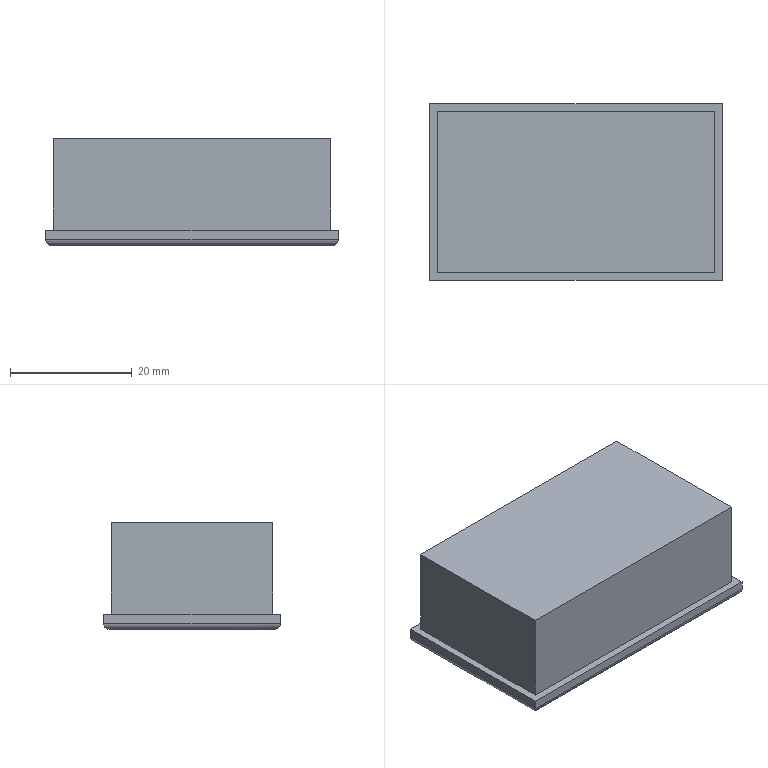Part | SolidWorks | features BaseBody 1 | 1 solid | 27 faces | box 48 x 29 x 17.5 mm | volume 19851 mm3 | plane 23 | cylinder 4 | commonest cylinder face diameters 2 x4
STEP:
#1=CARTESIAN_POINT('',(14.5,-5.,2.));
#2=VERTEX_POINT('',#1);
#3=CARTESIAN_POINT('',(12.5,-5.,2.));
#4=VERTEX_POINT('',#3);
#5=CARTESIAN_POINT('',(0.,-5.,2.));
#6=DIRECTION('',(-1.,0.,0.));
#7=VECTOR('',#6,1000.);
#8=LINE('',#5,#7);
#9=EDGE_CURVE('',#2,#4,#8,.T.);
#10=ORIENTED_EDGE('',*,*,#9,.T.);
#11=CARTESIAN_POINT('',(12.5,5.,2.));
#12=VERTEX_POINT('',#11);
#13=CARTESIAN_POINT('',(12.5,0.,2.));
#14=DIRECTION('',(0.,1.,0.));
#15=VECTOR('',#14,1000.);
#16=LINE('',#13,#15);
#17=EDGE_CURVE('',#4,#12,#16,.T.);
#18=ORIENTED_EDGE('',*,*,#17,.T.);
#19=CARTESIAN_POINT('',(14.5,5.,2.));
#20=VERTEX_POINT('',#19);
#21=CARTESIAN_POINT('',(0.,5.,2.));
#22=DIRECTION('',(1.,0.,0.));
#23=VECTOR('',#22,1000.);
#24=LINE('',#21,#23);
#25=EDGE_CURVE('',#12,#20,#24,.T.);
#26=ORIENTED_EDGE('',*,*,#25,.T.);
#27=CARTESIAN_POINT('',(14.5,0.,2.));
#28=DIRECTION('',(0.,-1.,0.));
#29=VECTOR('',#28,1000.);
#30=LINE('',#27,#29);
#31=EDGE_CURVE('',#20,#2,#30,.T.);
#32=ORIENTED_EDGE('',*,*,#31,.T.);
#33=EDGE_LOOP('',(#10,#18,#26,#32));
#34=FACE_OUTER_BOUND('',#33,.T.);
#35=CARTESIAN_POINT('',(0.,0.,2.));
#36=DIRECTION('',(0.,0.,1.));
#37=DIRECTION('',(1.,0.,0.));
#38=AXIS2_PLACEMENT_3D('',#35,#36,#37);
#39=PLANE('',#38);
#40=ADVANCED_FACE('',(#34),#39,.F.);
#41=CARTESIAN_POINT('',(-21.,11.5,0.));
#42=VERTEX_POINT('',#41);
#43=CARTESIAN_POINT('',(21.,11.5,0.));
#44=VERTEX_POINT('',#43);
#45=CARTESIAN_POINT('',(21.,11.5,0.));
#46=DIRECTION('',(1.,0.,0.));
#47=VECTOR('',#46,1000.);
#48=LINE('',#45,#47);
#49=EDGE_CURVE('',#42,#44,#48,.T.);
#50=ORIENTED_EDGE('',*,*,#49,.T.);
#51=CARTESIAN_POINT('',(19.,9.5,2.));
#52=VERTEX_POINT('',#51);
#53=CARTESIAN_POINT('',(21.,11.5,0.));
#54=DIRECTION('',(0.5774,0.5774,-0.5774));
#55=VECTOR('',#54,1000.);
#56=LINE('',#53,#55);
#57=EDGE_CURVE('',#52,#44,#56,.T.);
#58=ORIENTED_EDGE('',*,*,#57,.F.);
#59=CARTESIAN_POINT('',(-19.,9.5,2.));
#60=VERTEX_POINT('',#59);
#61=CARTESIAN_POINT('',(21.,9.5,2.));
#62=DIRECTION('',(1.,0.,0.));
#63=VECTOR('',#62,1000.);
#64=LINE('',#61,#63);
#65=EDGE_CURVE('',#60,#52,#64,.T.);
#66=ORIENTED_EDGE('',*,*,#65,.F.);
#67=CARTESIAN_POINT('',(-13.333,3.833,7.667));
#68=DIRECTION('',(-0.5774,0.5774,-0.5774));
#69=VECTOR('',#68,1000.);
#70=LINE('',#67,#69);
#71=EDGE_CURVE('',#60,#42,#70,.T.);
#72=ORIENTED_EDGE('',*,*,#71,.T.);
#73=EDGE_LOOP('',(#50,#58,#66,#72));
#74=FACE_OUTER_BOUND('',#73,.T.);
#75=CARTESIAN_POINT('',(21.,11.5,0.));
#76=DIRECTION('',(0.,0.7071,0.7071));
#77=DIRECTION('',(1.,0.,0.));
#78=AXIS2_PLACEMENT_3D('',#75,#76,#77);
#79=PLANE('',#78);
#80=ADVANCED_FACE('',(#74),#79,.F.);
#81=CARTESIAN_POINT('',(21.,-11.5,0.));
#82=VERTEX_POINT('',#81);
#83=CARTESIAN_POINT('',(21.,-11.5,0.));
#84=DIRECTION('',(0.,-1.,0.));
#85=VECTOR('',#84,1000.);
#86=LINE('',#83,#85);
#87=EDGE_CURVE('',#44,#82,#86,.T.);
#88=ORIENTED_EDGE('',*,*,#87,.T.);
#89=CARTESIAN_POINT('',(19.,-9.5,2.));
#90=VERTEX_POINT('',#89);
#91=CARTESIAN_POINT('',(21.,-11.5,0.));
#92=DIRECTION('',(0.5774,-0.5774,-0.5774));
#93=VECTOR('',#92,1000.);
#94=LINE('',#91,#93);
#95=EDGE_CURVE('',#90,#82,#94,.T.);
#96=ORIENTED_EDGE('',*,*,#95,.F.);
#97=CARTESIAN_POINT('',(19.,-11.5,2.));
#98=DIRECTION('',(0.,-1.,0.));
#99=VECTOR('',#98,1000.);
#100=LINE('',#97,#99);
#101=EDGE_CURVE('',#52,#90,#100,.T.);
#102=ORIENTED_EDGE('',*,*,#101,.F.);
#103=ORIENTED_EDGE('',*,*,#57,.T.);
#104=EDGE_LOOP('',(#88,#96,#102,#103));
#105=FACE_OUTER_BOUND('',#104,.T.);
#106=CARTESIAN_POINT('',(21.,-11.5,0.));
#107=DIRECTION('',(0.7071,0.,0.7071));
#108=DIRECTION('',(0.,-1.,0.));
#109=AXIS2_PLACEMENT_3D('',#106,#107,#108);
#110=PLANE('',#109);
#111=ADVANCED_FACE('',(#105),#110,.F.);
#112=CARTESIAN_POINT('',(-21.,-11.5,0.));
#113=VERTEX_POINT('',#112);
#114=CARTESIAN_POINT('',(21.,-11.5,0.));
#115=DIRECTION('',(-1.,0.,0.));
#116=VECTOR('',#115,1000.);
#117=LINE('',#114,#116);
#118=EDGE_CURVE('',#82,#113,#117,.T.);
#119=ORIENTED_EDGE('',*,*,#118,.T.);
#120=CARTESIAN_POINT('',(-19.,-9.5,2.));
#121=VERTEX_POINT('',#120);
#122=CARTESIAN_POINT('',(-7.,2.5,14.));
#123=DIRECTION('',(-0.5774,-0.5774,-0.5774));
#124=VECTOR('',#123,1000.);
#125=LINE('',#122,#124);
#126=EDGE_CURVE('',#121,#113,#125,.T.);
#127=ORIENTED_EDGE('',*,*,#126,.F.);
#128=CARTESIAN_POINT('',(21.,-9.5,2.));
#129=DIRECTION('',(-1.,0.,0.));
#130=VECTOR('',#129,1000.);
#131=LINE('',#128,#130);
#132=EDGE_CURVE('',#90,#121,#131,.T.);
#133=ORIENTED_EDGE('',*,*,#132,.F.);
#134=ORIENTED_EDGE('',*,*,#95,.T.);
#135=EDGE_LOOP('',(#119,#127,#133,#134));
#136=FACE_OUTER_BOUND('',#135,.T.);
#137=CARTESIAN_POINT('',(21.,-11.5,0.));
#138=DIRECTION('',(0.,-0.7071,0.7071));
#139=DIRECTION('',(-1.,0.,0.));
#140=AXIS2_PLACEMENT_3D('',#137,#138,#139);
#141=PLANE('',#140);
#142=ADVANCED_FACE('',(#136),#141,.F.);
#143=CARTESIAN_POINT('',(-21.,-11.5,0.));
#144=DIRECTION('',(0.,1.,0.));
#145=VECTOR('',#144,1000.);
#146=LINE('',#143,#145);
#147=EDGE_CURVE('',#113,#42,#146,.T.);
#148=ORIENTED_EDGE('',*,*,#147,.T.);
#149=ORIENTED_EDGE('',*,*,#71,.F.);
#150=CARTESIAN_POINT('',(-19.,-11.5,2.));
#151=DIRECTION('',(0.,1.,0.));
#152=VECTOR('',#151,1000.);
#153=LINE('',#150,#152);
#154=EDGE_CURVE('',#121,#60,#153,.T.);
#155=ORIENTED_EDGE('',*,*,#154,.F.);
#156=ORIENTED_EDGE('',*,*,#126,.T.);
#157=EDGE_LOOP('',(#148,#149,#155,#156));
#158=FACE_OUTER_BOUND('',#157,.T.);
#159=CARTESIAN_POINT('',(-21.,-11.5,0.));
#160=DIRECTION('',(-0.7071,0.,0.7071));
#161=DIRECTION('',(0.,1.,0.));
#162=AXIS2_PLACEMENT_3D('',#159,#160,#161);
#163=PLANE('',#162);
#164=ADVANCED_FACE('',(#158),#163,.F.);
#165=CARTESIAN_POINT('',(24.,-14.5,1.));
#166=VERTEX_POINT('',#165);
#167=CARTESIAN_POINT('',(23.,-13.5,0.));
#168=VERTEX_POINT('',#167);
#169=CARTESIAN_POINT('',(24.,-14.5,1.));
#170=CARTESIAN_POINT('',(24.,-14.5,0.4142));
#171=CARTESIAN_POINT('',(23.586,-14.086,0.));
#172=CARTESIAN_POINT('',(23.,-13.5,0.));
#173=(BOUNDED_CURVE()B_SPLINE_CURVE(3,(#169,#170,#171,#172),.UNSPECIFIED.,.F.,.T.)B_SPLINE_CURVE_WITH_KNOTS((4,4),(3.142,4.712),.UNSPECIFIED.)CURVE()GEOMETRIC_REPRESENTATION_ITEM()RATIONAL_B_SPLINE_CURVE((1.,0.8047,0.8047,1.))REPRESENTATION_ITEM(''));
#174=EDGE_CURVE('',#166,#168,#173,.T.);
#175=ORIENTED_EDGE('',*,*,#174,.T.);
#176=CARTESIAN_POINT('',(23.,13.5,0.));
#177=VERTEX_POINT('',#176);
#178=CARTESIAN_POINT('',(23.,-14.5,0.));
#179=DIRECTION('',(0.,-1.,0.));
#180=VECTOR('',#179,1000.);
#181=LINE('',#178,#180);
#182=EDGE_CURVE('',#177,#168,#181,.T.);
#183=ORIENTED_EDGE('',*,*,#182,.F.);
#184=CARTESIAN_POINT('',(24.,14.5,1.));
#185=VERTEX_POINT('',#184);
#186=CARTESIAN_POINT('',(23.,13.5,0.));
#187=CARTESIAN_POINT('',(23.586,14.086,0.));
#188=CARTESIAN_POINT('',(24.,14.5,0.4142));
#189=CARTESIAN_POINT('',(24.,14.5,1.));
#190=(BOUNDED_CURVE()B_SPLINE_CURVE(3,(#186,#187,#188,#189),.UNSPECIFIED.,.F.,.F.)B_SPLINE_CURVE_WITH_KNOTS((4,4),(4.712,6.283),.UNSPECIFIED.)CURVE()GEOMETRIC_REPRESENTATION_ITEM()RATIONAL_B_SPLINE_CURVE((1.,0.8047,0.8047,1.))REPRESENTATION_ITEM(''));
#191=EDGE_CURVE('',#177,#185,#190,.T.);
#192=ORIENTED_EDGE('',*,*,#191,.T.);
#193=CARTESIAN_POINT('',(24.,14.5,1.));
#194=DIRECTION('',(0.,1.,0.));
#195=VECTOR('',#194,1000.);
#196=LINE('',#193,#195);
#197=EDGE_CURVE('',#166,#185,#196,.T.);
#198=ORIENTED_EDGE('',*,*,#197,.F.);
#199=EDGE_LOOP('',(#175,#183,#192,#198));
#200=FACE_OUTER_BOUND('',#199,.T.);
#201=CARTESIAN_POINT('',(23.,-14.5,1.));
#202=DIRECTION('',(0.,-1.,0.));
#203=DIRECTION('',(0.,0.,-1.));
#204=AXIS2_PLACEMENT_3D('',#201,#202,#203);
#205=CYLINDRICAL_SURFACE('',#204,1.);
#206=ADVANCED_FACE('',(#200),#205,.T.);
#207=CARTESIAN_POINT('',(-23.,13.5,0.));
#208=VERTEX_POINT('',#207);
#209=CARTESIAN_POINT('',(-24.,14.5,1.));
#210=VERTEX_POINT('',#209);
#211=CARTESIAN_POINT('',(-23.,13.5,0.));
#212=CARTESIAN_POINT('',(-23.586,14.086,0.));
#213=CARTESIAN_POINT('',(-24.,14.5,0.4142));
#214=CARTESIAN_POINT('',(-24.,14.5,1.));
#215=(BOUNDED_CURVE()B_SPLINE_CURVE(3,(#211,#212,#213,#214),.UNSPECIFIED.,.F.,.T.)B_SPLINE_CURVE_WITH_KNOTS((4,4),(1.571,3.142),.UNSPECIFIED.)CURVE()GEOMETRIC_REPRESENTATION_ITEM()RATIONAL_B_SPLINE_CURVE((1.,0.8047,0.8047,1.))REPRESENTATION_ITEM(''));
#216=EDGE_CURVE('',#208,#210,#215,.T.);
#217=ORIENTED_EDGE('',*,*,#216,.T.);
#218=CARTESIAN_POINT('',(-24.,14.5,1.));
#219=DIRECTION('',(-1.,0.,0.));
#220=VECTOR('',#219,1000.);
#221=LINE('',#218,#220);
#222=EDGE_CURVE('',#185,#210,#221,.T.);
#223=ORIENTED_EDGE('',*,*,#222,.F.);
#224=ORIENTED_EDGE('',*,*,#191,.F.);
#225=CARTESIAN_POINT('',(24.,13.5,0.));
#226=DIRECTION('',(1.,0.,0.));
#227=VECTOR('',#226,1000.);
#228=LINE('',#225,#227);
#229=EDGE_CURVE('',#208,#177,#228,.T.);
#230=ORIENTED_EDGE('',*,*,#229,.F.);
#231=EDGE_LOOP('',(#217,#223,#224,#230));
#232=FACE_OUTER_BOUND('',#231,.T.);
#233=CARTESIAN_POINT('',(-24.,13.5,1.));
#234=DIRECTION('',(1.,0.,0.));
#235=DIRECTION('',(0.,0.,-1.));
#236=AXIS2_PLACEMENT_3D('',#233,#234,#235);
#237=CYLINDRICAL_SURFACE('',#236,1.);
#238=ADVANCED_FACE('',(#232),#237,.T.);
#239=CARTESIAN_POINT('',(-24.,-14.5,1.));
#240=VERTEX_POINT('',#239);
#241=CARTESIAN_POINT('',(-23.,-13.5,0.));
#242=VERTEX_POINT('',#241);
#243=CARTESIAN_POINT('',(-24.,-14.5,1.));
#244=CARTESIAN_POINT('',(-24.,-14.5,0.4142));
#245=CARTESIAN_POINT('',(-23.586,-14.086,0.));
#246=CARTESIAN_POINT('',(-23.,-13.5,0.));
#247=(BOUNDED_CURVE()B_SPLINE_CURVE(3,(#243,#244,#245,#246),.UNSPECIFIED.,.F.,.F.)B_SPLINE_CURVE_WITH_KNOTS((4,4),(3.142,4.712),.UNSPECIFIED.)CURVE()GEOMETRIC_REPRESENTATION_ITEM()RATIONAL_B_SPLINE_CURVE((1.,0.8047,0.8047,1.))REPRESENTATION_ITEM(''));
#248=EDGE_CURVE('',#240,#242,#247,.T.);
#249=ORIENTED_EDGE('',*,*,#248,.T.);
#250=CARTESIAN_POINT('',(-24.,-13.5,0.));
#251=DIRECTION('',(-1.,0.,0.));
#252=VECTOR('',#251,1000.);
#253=LINE('',#250,#252);
#254=EDGE_CURVE('',#168,#242,#253,.T.);
#255=ORIENTED_EDGE('',*,*,#254,.F.);
#256=ORIENTED_EDGE('',*,*,#174,.F.);
#257=CARTESIAN_POINT('',(24.,-14.5,1.));
#258=DIRECTION('',(1.,0.,0.));
#259=VECTOR('',#258,1000.);
#260=LINE('',#257,#259);
#261=EDGE_CURVE('',#240,#166,#260,.T.);
#262=ORIENTED_EDGE('',*,*,#261,.F.);
#263=EDGE_LOOP('',(#249,#255,#256,#262));
#264=FACE_OUTER_BOUND('',#263,.T.);
#265=CARTESIAN_POINT('',(-24.,-13.5,1.));
#266=DIRECTION('',(-1.,0.,0.));
#267=DIRECTION('',(0.,0.,1.));
#268=AXIS2_PLACEMENT_3D('',#265,#266,#267);
#269=CYLINDRICAL_SURFACE('',#268,1.);
#270=ADVANCED_FACE('',(#264),#269,.T.);
#271=ORIENTED_EDGE('',*,*,#216,.F.);
#272=CARTESIAN_POINT('',(-23.,14.5,0.));
#273=DIRECTION('',(0.,1.,0.));
#274=VECTOR('',#273,1000.);
#275=LINE('',#272,#274);
#276=EDGE_CURVE('',#242,#208,#275,.T.);
#277=ORIENTED_EDGE('',*,*,#276,.F.);
#278=ORIENTED_EDGE('',*,*,#248,.F.);
#279=CARTESIAN_POINT('',(-24.,-14.5,1.));
#280=DIRECTION('',(0.,-1.,0.));
#281=VECTOR('',#280,1000.);
#282=LINE('',#279,#281);
#283=EDGE_CURVE('',#210,#240,#282,.T.);
#284=ORIENTED_EDGE('',*,*,#283,.F.);
#285=EDGE_LOOP('',(#271,#277,#278,#284));
#286=FACE_OUTER_BOUND('',#285,.T.);
#287=CARTESIAN_POINT('',(-23.,-14.5,1.));
#288=DIRECTION('',(0.,1.,0.));
#289=DIRECTION('',(0.,0.,1.));
#290=AXIS2_PLACEMENT_3D('',#287,#288,#289);
#291=CYLINDRICAL_SURFACE('',#290,1.);
#292=ADVANCED_FACE('',(#286),#291,.T.);
#293=CARTESIAN_POINT('',(22.75,-13.25,17.5));
#294=VERTEX_POINT('',#293);
#295=CARTESIAN_POINT('',(22.75,13.25,17.5));
#296=VERTEX_POINT('',#295);
#297=CARTESIAN_POINT('',(22.75,-13.25,17.5));
#298=DIRECTION('',(0.,1.,0.));
#299=VECTOR('',#298,1000.);
#300=LINE('',#297,#299);
#301=EDGE_CURVE('',#294,#296,#300,.T.);
#302=ORIENTED_EDGE('',*,*,#301,.T.);
#303=CARTESIAN_POINT('',(-22.75,13.25,17.5));
#304=VERTEX_POINT('',#303);
#305=CARTESIAN_POINT('',(-22.75,13.25,17.5));
#306=DIRECTION('',(-1.,0.,0.));
#307=VECTOR('',#306,1000.);
#308=LINE('',#305,#307);
#309=EDGE_CURVE('',#296,#304,#308,.T.);
#310=ORIENTED_EDGE('',*,*,#309,.T.);
#311=CARTESIAN_POINT('',(-22.75,-13.25,17.5));
#312=VERTEX_POINT('',#311);
#313=CARTESIAN_POINT('',(-22.75,-13.25,17.5));
#314=DIRECTION('',(0.,-1.,0.));
#315=VECTOR('',#314,1000.);
#316=LINE('',#313,#315);
#317=EDGE_CURVE('',#304,#312,#316,.T.);
#318=ORIENTED_EDGE('',*,*,#317,.T.);
#319=CARTESIAN_POINT('',(-22.75,-13.25,17.5));
#320=DIRECTION('',(1.,0.,0.));
#321=VECTOR('',#320,1000.);
#322=LINE('',#319,#321);
#323=EDGE_CURVE('',#312,#294,#322,.T.);
#324=ORIENTED_EDGE('',*,*,#323,.T.);
#325=EDGE_LOOP('',(#302,#310,#318,#324));
#326=FACE_OUTER_BOUND('',#325,.T.);
#327=CARTESIAN_POINT('',(0.,0.,17.5));
#328=DIRECTION('',(0.,0.,-1.));
#329=DIRECTION('',(0.,-1.,0.));
#330=AXIS2_PLACEMENT_3D('',#327,#328,#329);
#331=PLANE('',#330);
#332=ADVANCED_FACE('',(#326),#331,.F.);
#333=CARTESIAN_POINT('',(-22.75,-13.25,2.5));
#334=VERTEX_POINT('',#333);
#335=CARTESIAN_POINT('',(22.75,-13.25,2.5));
#336=VERTEX_POINT('',#335);
#337=CARTESIAN_POINT('',(-22.75,-13.25,2.5));
#338=DIRECTION('',(1.,0.,0.));
#339=VECTOR('',#338,1000.);
#340=LINE('',#337,#339);
#341=EDGE_CURVE('',#334,#336,#340,.T.);
#342=ORIENTED_EDGE('',*,*,#341,.T.);
#343=CARTESIAN_POINT('',(22.75,-13.25,17.5));
#344=DIRECTION('',(0.,0.,-1.));
#345=VECTOR('',#344,1000.);
#346=LINE('',#343,#345);
#347=EDGE_CURVE('',#294,#336,#346,.T.);
#348=ORIENTED_EDGE('',*,*,#347,.F.);
#349=ORIENTED_EDGE('',*,*,#323,.F.);
#350=CARTESIAN_POINT('',(-22.75,-13.25,17.5));
#351=DIRECTION('',(0.,0.,-1.));
#352=VECTOR('',#351,1000.);
#353=LINE('',#350,#352);
#354=EDGE_CURVE('',#312,#334,#353,.T.);
#355=ORIENTED_EDGE('',*,*,#354,.T.);
#356=EDGE_LOOP('',(#342,#348,#349,#355));
#357=FACE_OUTER_BOUND('',#356,.T.);
#358=CARTESIAN_POINT('',(-22.75,-13.25,17.5));
#359=DIRECTION('',(0.,1.,0.));
#360=DIRECTION('',(1.,0.,0.));
#361=AXIS2_PLACEMENT_3D('',#358,#359,#360);
#362=PLANE('',#361);
#363=ADVANCED_FACE('',(#357),#362,.F.);
#364=CARTESIAN_POINT('',(-22.75,13.25,2.5));
#365=VERTEX_POINT('',#364);
#366=CARTESIAN_POINT('',(-22.75,-13.25,2.5));
#367=DIRECTION('',(0.,-1.,0.));
#368=VECTOR('',#367,1000.);
#369=LINE('',#366,#368);
#370=EDGE_CURVE('',#365,#334,#369,.T.);
#371=ORIENTED_EDGE('',*,*,#370,.T.);
#372=ORIENTED_EDGE('',*,*,#354,.F.);
#373=ORIENTED_EDGE('',*,*,#317,.F.);
#374=CARTESIAN_POINT('',(-22.75,13.25,17.5));
#375=DIRECTION('',(0.,0.,-1.));
#376=VECTOR('',#375,1000.);
#377=LINE('',#374,#376);
#378=EDGE_CURVE('',#304,#365,#377,.T.);
#379=ORIENTED_EDGE('',*,*,#378,.T.);
#380=EDGE_LOOP('',(#371,#372,#373,#379));
#381=FACE_OUTER_BOUND('',#380,.T.);
#382=CARTESIAN_POINT('',(-22.75,-13.25,17.5));
#383=DIRECTION('',(1.,0.,0.));
#384=DIRECTION('',(0.,1.,0.));
#385=AXIS2_PLACEMENT_3D('',#382,#383,#384);
#386=PLANE('',#385);
#387=ADVANCED_FACE('',(#381),#386,.F.);
#388=CARTESIAN_POINT('',(22.75,13.25,2.5));
#389=VERTEX_POINT('',#388);
#390=CARTESIAN_POINT('',(-22.75,13.25,2.5));
#391=DIRECTION('',(-1.,0.,0.));
#392=VECTOR('',#391,1000.);
#393=LINE('',#390,#392);
#394=EDGE_CURVE('',#389,#365,#393,.T.);
#395=ORIENTED_EDGE('',*,*,#394,.T.);
#396=ORIENTED_EDGE('',*,*,#378,.F.);
#397=ORIENTED_EDGE('',*,*,#309,.F.);
#398=CARTESIAN_POINT('',(22.75,13.25,17.5));
#399=DIRECTION('',(0.,0.,-1.));
#400=VECTOR('',#399,1000.);
#401=LINE('',#398,#400);
#402=EDGE_CURVE('',#296,#389,#401,.T.);
#403=ORIENTED_EDGE('',*,*,#402,.T.);
#404=EDGE_LOOP('',(#395,#396,#397,#403));
#405=FACE_OUTER_BOUND('',#404,.T.);
#406=CARTESIAN_POINT('',(-22.75,13.25,17.5));
#407=DIRECTION('',(0.,-1.,0.));
#408=DIRECTION('',(0.,0.,-1.));
#409=AXIS2_PLACEMENT_3D('',#406,#407,#408);
#410=PLANE('',#409);
#411=ADVANCED_FACE('',(#405),#410,.F.);
#412=CARTESIAN_POINT('',(22.75,-13.25,2.5));
#413=DIRECTION('',(0.,1.,0.));
#414=VECTOR('',#413,1000.);
#415=LINE('',#412,#414);
#416=EDGE_CURVE('',#336,#389,#415,.T.);
#417=ORIENTED_EDGE('',*,*,#416,.T.);
#418=ORIENTED_EDGE('',*,*,#402,.F.);
#419=ORIENTED_EDGE('',*,*,#301,.F.);
#420=ORIENTED_EDGE('',*,*,#347,.T.);
#421=EDGE_LOOP('',(#417,#418,#419,#420));
#422=FACE_OUTER_BOUND('',#421,.T.);
#423=CARTESIAN_POINT('',(22.75,-13.25,17.5));
#424=DIRECTION('',(-1.,0.,0.));
#425=DIRECTION('',(0.,0.,1.));
#426=AXIS2_PLACEMENT_3D('',#423,#424,#425);
#427=PLANE('',#426);
#428=ADVANCED_FACE('',(#422),#427,.F.);
#429=ORIENTED_EDGE('',*,*,#147,.F.);
#430=ORIENTED_EDGE('',*,*,#118,.F.);
#431=ORIENTED_EDGE('',*,*,#87,.F.);
#432=ORIENTED_EDGE('',*,*,#49,.F.);
#433=EDGE_LOOP('',(#429,#430,#431,#432));
#434=FACE_BOUND('',#433,.T.);
#435=ORIENTED_EDGE('',*,*,#229,.T.);
#436=ORIENTED_EDGE('',*,*,#182,.T.);
#437=ORIENTED_EDGE('',*,*,#254,.T.);
#438=ORIENTED_EDGE('',*,*,#276,.T.);
#439=EDGE_LOOP('',(#435,#436,#437,#438));
#440=FACE_OUTER_BOUND('',#439,.T.);
#441=CARTESIAN_POINT('',(0.,0.,0.));
#442=DIRECTION('',(0.,0.,-1.));
#443=DIRECTION('',(0.,-1.,0.));
#444=AXIS2_PLACEMENT_3D('',#441,#442,#443);
#445=PLANE('',#444);
#446=ADVANCED_FACE('',(#434,#440),#445,.T.);
#447=CARTESIAN_POINT('',(-24.,-14.5,2.5));
#448=VERTEX_POINT('',#447);
#449=CARTESIAN_POINT('',(-24.,-14.5,2.5));
#450=DIRECTION('',(0.,0.,-1.));
#451=VECTOR('',#450,1000.);
#452=LINE('',#449,#451);
#453=EDGE_CURVE('',#448,#240,#452,.T.);
#454=ORIENTED_EDGE('',*,*,#453,.T.);
#455=ORIENTED_EDGE('',*,*,#261,.T.);
#456=CARTESIAN_POINT('',(24.,-14.5,2.5));
#457=VERTEX_POINT('',#456);
#458=CARTESIAN_POINT('',(24.,-14.5,2.5));
#459=DIRECTION('',(0.,0.,-1.));
#460=VECTOR('',#459,1000.);
#461=LINE('',#458,#460);
#462=EDGE_CURVE('',#457,#166,#461,.T.);
#463=ORIENTED_EDGE('',*,*,#462,.F.);
#464=CARTESIAN_POINT('',(-24.,-14.5,2.5));
#465=DIRECTION('',(1.,0.,0.));
#466=VECTOR('',#465,1000.);
#467=LINE('',#464,#466);
#468=EDGE_CURVE('',#448,#457,#467,.T.);
#469=ORIENTED_EDGE('',*,*,#468,.F.);
#470=EDGE_LOOP('',(#454,#455,#463,#469));
#471=FACE_OUTER_BOUND('',#470,.T.);
#472=CARTESIAN_POINT('',(-24.,-14.5,2.5));
#473=DIRECTION('',(0.,1.,0.));
#474=DIRECTION('',(1.,0.,0.));
#475=AXIS2_PLACEMENT_3D('',#472,#473,#474);
#476=PLANE('',#475);
#477=ADVANCED_FACE('',(#471),#476,.F.);
#478=CARTESIAN_POINT('',(-24.,14.5,2.5));
#479=VERTEX_POINT('',#478);
#480=CARTESIAN_POINT('',(-24.,14.5,2.5));
#481=DIRECTION('',(0.,0.,-1.));
#482=VECTOR('',#481,1000.);
#483=LINE('',#480,#482);
#484=EDGE_CURVE('',#479,#210,#483,.T.);
#485=ORIENTED_EDGE('',*,*,#484,.T.);
#486=ORIENTED_EDGE('',*,*,#283,.T.);
#487=ORIENTED_EDGE('',*,*,#453,.F.);
#488=CARTESIAN_POINT('',(-24.,-14.5,2.5));
#489=DIRECTION('',(0.,-1.,0.));
#490=VECTOR('',#489,1000.);
#491=LINE('',#488,#490);
#492=EDGE_CURVE('',#479,#448,#491,.T.);
#493=ORIENTED_EDGE('',*,*,#492,.F.);
#494=EDGE_LOOP('',(#485,#486,#487,#493));
#495=FACE_OUTER_BOUND('',#494,.T.);
#496=CARTESIAN_POINT('',(-24.,-14.5,2.5));
#497=DIRECTION('',(1.,0.,0.));
#498=DIRECTION('',(0.,1.,0.));
#499=AXIS2_PLACEMENT_3D('',#496,#497,#498);
#500=PLANE('',#499);
#501=ADVANCED_FACE('',(#495),#500,.F.);
#502=CARTESIAN_POINT('',(24.,14.5,2.5));
#503=VERTEX_POINT('',#502);
#504=CARTESIAN_POINT('',(24.,14.5,2.5));
#505=DIRECTION('',(0.,0.,-1.));
#506=VECTOR('',#505,1000.);
#507=LINE('',#504,#506);
#508=EDGE_CURVE('',#503,#185,#507,.T.);
#509=ORIENTED_EDGE('',*,*,#508,.T.);
#510=ORIENTED_EDGE('',*,*,#222,.T.);
#511=ORIENTED_EDGE('',*,*,#484,.F.);
#512=CARTESIAN_POINT('',(-24.,14.5,2.5));
#513=DIRECTION('',(-1.,0.,0.));
#514=VECTOR('',#513,1000.);
#515=LINE('',#512,#514);
#516=EDGE_CURVE('',#503,#479,#515,.T.);
#517=ORIENTED_EDGE('',*,*,#516,.F.);
#518=EDGE_LOOP('',(#509,#510,#511,#517));
#519=FACE_OUTER_BOUND('',#518,.T.);
#520=CARTESIAN_POINT('',(-24.,14.5,2.5));
#521=DIRECTION('',(0.,-1.,0.));
#522=DIRECTION('',(0.,0.,-1.));
#523=AXIS2_PLACEMENT_3D('',#520,#521,#522);
#524=PLANE('',#523);
#525=ADVANCED_FACE('',(#519),#524,.F.);
#526=ORIENTED_EDGE('',*,*,#462,.T.);
#527=ORIENTED_EDGE('',*,*,#197,.T.);
#528=ORIENTED_EDGE('',*,*,#508,.F.);
#529=CARTESIAN_POINT('',(24.,-14.5,2.5));
#530=DIRECTION('',(0.,1.,0.));
#531=VECTOR('',#530,1000.);
#532=LINE('',#529,#531);
#533=EDGE_CURVE('',#457,#503,#532,.T.);
#534=ORIENTED_EDGE('',*,*,#533,.F.);
#535=EDGE_LOOP('',(#526,#527,#528,#534));
#536=FACE_OUTER_BOUND('',#535,.T.);
#537=CARTESIAN_POINT('',(24.,-14.5,2.5));
#538=DIRECTION('',(-1.,0.,0.));
#539=DIRECTION('',(0.,0.,1.));
#540=AXIS2_PLACEMENT_3D('',#537,#538,#539);
#541=PLANE('',#540);
#542=ADVANCED_FACE('',(#536),#541,.F.);
#543=ORIENTED_EDGE('',*,*,#416,.F.);
#544=ORIENTED_EDGE('',*,*,#341,.F.);
#545=ORIENTED_EDGE('',*,*,#370,.F.);
#546=ORIENTED_EDGE('',*,*,#394,.F.);
#547=EDGE_LOOP('',(#543,#544,#545,#546));
#548=FACE_BOUND('',#547,.T.);
#549=ORIENTED_EDGE('',*,*,#533,.T.);
#550=ORIENTED_EDGE('',*,*,#516,.T.);
#551=ORIENTED_EDGE('',*,*,#492,.T.);
#552=ORIENTED_EDGE('',*,*,#468,.T.);
#553=EDGE_LOOP('',(#549,#550,#551,#552));
#554=FACE_OUTER_BOUND('',#553,.T.);
#555=CARTESIAN_POINT('',(0.,0.,2.5));
#556=DIRECTION('',(0.,0.,-1.));
#557=DIRECTION('',(0.,-1.,0.));
#558=AXIS2_PLACEMENT_3D('',#555,#556,#557);
#559=PLANE('',#558);
#560=ADVANCED_FACE('',(#548,#554),#559,.F.);
#561=CARTESIAN_POINT('',(8.5,-5.,2.));
#562=VERTEX_POINT('',#561);
#563=CARTESIAN_POINT('',(8.5,5.,2.));
#564=VERTEX_POINT('',#563);
#565=CARTESIAN_POINT('',(8.5,0.,2.));
#566=DIRECTION('',(0.,1.,0.));
#567=VECTOR('',#566,1000.);
#568=LINE('',#565,#567);
#569=EDGE_CURVE('',#562,#564,#568,.T.);
#570=ORIENTED_EDGE('',*,*,#569,.T.);
#571=CARTESIAN_POINT('',(10.5,5.,2.));
#572=VERTEX_POINT('',#571);
#573=CARTESIAN_POINT('',(0.,5.,2.));
#574=DIRECTION('',(1.,0.,0.));
#575=VECTOR('',#574,1000.);
#576=LINE('',#573,#575);
#577=EDGE_CURVE('',#564,#572,#576,.T.);
#578=ORIENTED_EDGE('',*,*,#577,.T.);
#579=CARTESIAN_POINT('',(10.5,-5.,2.));
#580=VERTEX_POINT('',#579);
#581=CARTESIAN_POINT('',(10.5,0.,2.));
#582=DIRECTION('',(0.,-1.,0.));
#583=VECTOR('',#582,1000.);
#584=LINE('',#581,#583);
#585=EDGE_CURVE('',#572,#580,#584,.T.);
#586=ORIENTED_EDGE('',*,*,#585,.T.);
#587=CARTESIAN_POINT('',(0.,-5.,2.));
#588=DIRECTION('',(-1.,0.,0.));
#589=VECTOR('',#588,1000.);
#590=LINE('',#587,#589);
#591=EDGE_CURVE('',#580,#562,#590,.T.);
#592=ORIENTED_EDGE('',*,*,#591,.T.);
#593=EDGE_LOOP('',(#570,#578,#586,#592));
#594=FACE_OUTER_BOUND('',#593,.T.);
#595=CARTESIAN_POINT('',(0.,0.,2.));
#596=DIRECTION('',(0.,0.,1.));
#597=DIRECTION('',(1.,0.,0.));
#598=AXIS2_PLACEMENT_3D('',#595,#596,#597);
#599=PLANE('',#598);
#600=ADVANCED_FACE('',(#594),#599,.F.);
#601=CARTESIAN_POINT('',(16.,6.5,2.));
#602=VERTEX_POINT('',#601);
#603=CARTESIAN_POINT('',(16.,-6.5,2.));
#604=VERTEX_POINT('',#603);
#605=CARTESIAN_POINT('',(16.,0.,2.));
#606=DIRECTION('',(0.,-1.,0.));
#607=VECTOR('',#606,1000.);
#608=LINE('',#605,#607);
#609=EDGE_CURVE('',#602,#604,#608,.T.);
#610=ORIENTED_EDGE('',*,*,#609,.F.);
#611=CARTESIAN_POINT('',(-13.5,6.5,2.));
#612=VERTEX_POINT('',#611);
#613=CARTESIAN_POINT('',(0.,6.5,2.));
#614=DIRECTION('',(1.,0.,0.));
#615=VECTOR('',#614,1000.);
#616=LINE('',#613,#615);
#617=EDGE_CURVE('',#612,#602,#616,.T.);
#618=ORIENTED_EDGE('',*,*,#617,.F.);
#619=CARTESIAN_POINT('',(-13.5,-6.5,2.));
#620=VERTEX_POINT('',#619);
#621=CARTESIAN_POINT('',(-13.5,0.,2.));
#622=DIRECTION('',(0.,1.,0.));
#623=VECTOR('',#622,1000.);
#624=LINE('',#621,#623);
#625=EDGE_CURVE('',#620,#612,#624,.T.);
#626=ORIENTED_EDGE('',*,*,#625,.F.);
#627=CARTESIAN_POINT('',(0.,-6.5,2.));
#628=DIRECTION('',(-1.,0.,0.));
#629=VECTOR('',#628,1000.);
#630=LINE('',#627,#629);
#631=EDGE_CURVE('',#604,#620,#630,.T.);
#632=ORIENTED_EDGE('',*,*,#631,.F.);
#633=EDGE_LOOP('',(#610,#618,#626,#632));
#634=FACE_BOUND('',#633,.T.);
#635=CARTESIAN_POINT('',(-15.,2.5,2.));
#636=VERTEX_POINT('',#635);
#637=CARTESIAN_POINT('',(-15.,8.,2.));
#638=VERTEX_POINT('',#637);
#639=CARTESIAN_POINT('',(-15.,0.,2.));
#640=DIRECTION('',(0.,1.,0.));
#641=VECTOR('',#640,1000.);
#642=LINE('',#639,#641);
#643=EDGE_CURVE('',#636,#638,#642,.T.);
#644=ORIENTED_EDGE('',*,*,#643,.T.);
#645=CARTESIAN_POINT('',(17.5,8.,2.));
#646=VERTEX_POINT('',#645);
#647=CARTESIAN_POINT('',(0.,8.,2.));
#648=DIRECTION('',(1.,0.,0.));
#649=VECTOR('',#648,1000.);
#650=LINE('',#647,#649);
#651=EDGE_CURVE('',#638,#646,#650,.T.);
#652=ORIENTED_EDGE('',*,*,#651,.T.);
#653=CARTESIAN_POINT('',(17.5,-8.,2.));
#654=VERTEX_POINT('',#653);
#655=CARTESIAN_POINT('',(17.5,0.,2.));
#656=DIRECTION('',(0.,-1.,0.));
#657=VECTOR('',#656,1000.);
#658=LINE('',#655,#657);
#659=EDGE_CURVE('',#646,#654,#658,.T.);
#660=ORIENTED_EDGE('',*,*,#659,.T.);
#661=CARTESIAN_POINT('',(-15.,-8.,2.));
#662=VERTEX_POINT('',#661);
#663=CARTESIAN_POINT('',(0.,-8.,2.));
#664=DIRECTION('',(-1.,0.,0.));
#665=VECTOR('',#664,1000.);
#666=LINE('',#663,#665);
#667=EDGE_CURVE('',#654,#662,#666,.T.);
#668=ORIENTED_EDGE('',*,*,#667,.T.);
#669=CARTESIAN_POINT('',(-15.,-2.5,2.));
#670=VERTEX_POINT('',#669);
#671=CARTESIAN_POINT('',(-15.,0.,2.));
#672=DIRECTION('',(0.,1.,0.));
#673=VECTOR('',#672,1000.);
#674=LINE('',#671,#673);
#675=EDGE_CURVE('',#662,#670,#674,.T.);
#676=ORIENTED_EDGE('',*,*,#675,.T.);
#677=CARTESIAN_POINT('',(-17.,-2.5,2.));
#678=VERTEX_POINT('',#677);
#679=CARTESIAN_POINT('',(0.,-2.5,2.));
#680=DIRECTION('',(-1.,0.,0.));
#681=VECTOR('',#680,1000.);
#682=LINE('',#679,#681);
#683=EDGE_CURVE('',#670,#678,#682,.T.);
#684=ORIENTED_EDGE('',*,*,#683,.T.);
#685=CARTESIAN_POINT('',(-17.,2.5,2.));
#686=VERTEX_POINT('',#685);
#687=CARTESIAN_POINT('',(-17.,0.,2.));
#688=DIRECTION('',(0.,1.,0.));
#689=VECTOR('',#688,1000.);
#690=LINE('',#687,#689);
#691=EDGE_CURVE('',#678,#686,#690,.T.);
#692=ORIENTED_EDGE('',*,*,#691,.T.);
#693=CARTESIAN_POINT('',(0.,2.5,2.));
#694=DIRECTION('',(1.,0.,0.));
#695=VECTOR('',#694,1000.);
#696=LINE('',#693,#695);
#697=EDGE_CURVE('',#686,#636,#696,.T.);
#698=ORIENTED_EDGE('',*,*,#697,.T.);
#699=EDGE_LOOP('',(#644,#652,#660,#668,#676,#684,#692,#698));
#700=FACE_OUTER_BOUND('',#699,.T.);
#701=CARTESIAN_POINT('',(0.,0.,2.));
#702=DIRECTION('',(0.,0.,1.));
#703=DIRECTION('',(1.,0.,0.));
#704=AXIS2_PLACEMENT_3D('',#701,#702,#703);
#705=PLANE('',#704);
#706=ADVANCED_FACE('',(#634,#700),#705,.F.);
#707=CARTESIAN_POINT('',(4.5,-5.,2.));
#708=VERTEX_POINT('',#707);
#709=CARTESIAN_POINT('',(4.5,5.,2.));
#710=VERTEX_POINT('',#709);
#711=CARTESIAN_POINT('',(4.5,0.,2.));
#712=DIRECTION('',(0.,1.,0.));
#713=VECTOR('',#712,1000.);
#714=LINE('',#711,#713);
#715=EDGE_CURVE('',#708,#710,#714,.T.);
#716=ORIENTED_EDGE('',*,*,#715,.T.);
#717=CARTESIAN_POINT('',(6.5,5.,2.));
#718=VERTEX_POINT('',#717);
#719=CARTESIAN_POINT('',(0.,5.,2.));
#720=DIRECTION('',(1.,0.,0.));
#721=VECTOR('',#720,1000.);
#722=LINE('',#719,#721);
#723=EDGE_CURVE('',#710,#718,#722,.T.);
#724=ORIENTED_EDGE('',*,*,#723,.T.);
#725=CARTESIAN_POINT('',(6.5,-5.,2.));
#726=VERTEX_POINT('',#725);
#727=CARTESIAN_POINT('',(6.5,0.,2.));
#728=DIRECTION('',(0.,-1.,0.));
#729=VECTOR('',#728,1000.);
#730=LINE('',#727,#729);
#731=EDGE_CURVE('',#718,#726,#730,.T.);
#732=ORIENTED_EDGE('',*,*,#731,.T.);
#733=CARTESIAN_POINT('',(0.,-5.,2.));
#734=DIRECTION('',(-1.,0.,0.));
#735=VECTOR('',#734,1000.);
#736=LINE('',#733,#735);
#737=EDGE_CURVE('',#726,#708,#736,.T.);
#738=ORIENTED_EDGE('',*,*,#737,.T.);
#739=EDGE_LOOP('',(#716,#724,#732,#738));
#740=FACE_OUTER_BOUND('',#739,.T.);
#741=CARTESIAN_POINT('',(0.,0.,2.));
#742=DIRECTION('',(0.,0.,1.));
#743=DIRECTION('',(1.,0.,0.));
#744=AXIS2_PLACEMENT_3D('',#741,#742,#743);
#745=PLANE('',#744);
#746=ADVANCED_FACE('',(#740),#745,.F.);
#747=CARTESIAN_POINT('',(0.5,-5.,2.));
#748=VERTEX_POINT('',#747);
#749=CARTESIAN_POINT('',(0.5,5.,2.));
#750=VERTEX_POINT('',#749);
#751=CARTESIAN_POINT('',(0.5,0.,2.));
#752=DIRECTION('',(0.,1.,0.));
#753=VECTOR('',#752,1000.);
#754=LINE('',#751,#753);
#755=EDGE_CURVE('',#748,#750,#754,.T.);
#756=ORIENTED_EDGE('',*,*,#755,.T.);
#757=CARTESIAN_POINT('',(2.5,5.,2.));
#758=VERTEX_POINT('',#757);
#759=CARTESIAN_POINT('',(0.,5.,2.));
#760=DIRECTION('',(1.,0.,0.));
#761=VECTOR('',#760,1000.);
#762=LINE('',#759,#761);
#763=EDGE_CURVE('',#750,#758,#762,.T.);
#764=ORIENTED_EDGE('',*,*,#763,.T.);
#765=CARTESIAN_POINT('',(2.5,-5.,2.));
#766=VERTEX_POINT('',#765);
#767=CARTESIAN_POINT('',(2.5,0.,2.));
#768=DIRECTION('',(0.,-1.,0.));
#769=VECTOR('',#768,1000.);
#770=LINE('',#767,#769);
#771=EDGE_CURVE('',#758,#766,#770,.T.);
#772=ORIENTED_EDGE('',*,*,#771,.T.);
#773=CARTESIAN_POINT('',(0.,-5.,2.));
#774=DIRECTION('',(-1.,0.,0.));
#775=VECTOR('',#774,1000.);
#776=LINE('',#773,#775);
#777=EDGE_CURVE('',#766,#748,#776,.T.);
#778=ORIENTED_EDGE('',*,*,#777,.T.);
#779=EDGE_LOOP('',(#756,#764,#772,#778));
#780=FACE_OUTER_BOUND('',#779,.T.);
#781=CARTESIAN_POINT('',(0.,0.,2.));
#782=DIRECTION('',(0.,0.,1.));
#783=DIRECTION('',(1.,0.,0.));
#784=AXIS2_PLACEMENT_3D('',#781,#782,#783);
#785=PLANE('',#784);
#786=ADVANCED_FACE('',(#780),#785,.F.);
#787=CARTESIAN_POINT('',(-3.5,-5.,2.));
#788=VERTEX_POINT('',#787);
#789=CARTESIAN_POINT('',(-3.5,5.,2.));
#790=VERTEX_POINT('',#789);
#791=CARTESIAN_POINT('',(-3.5,0.,2.));
#792=DIRECTION('',(0.,1.,0.));
#793=VECTOR('',#792,1000.);
#794=LINE('',#791,#793);
#795=EDGE_CURVE('',#788,#790,#794,.T.);
#796=ORIENTED_EDGE('',*,*,#795,.T.);
#797=CARTESIAN_POINT('',(-1.5,5.,2.));
#798=VERTEX_POINT('',#797);
#799=CARTESIAN_POINT('',(0.,5.,2.));
#800=DIRECTION('',(1.,0.,0.));
#801=VECTOR('',#800,1000.);
#802=LINE('',#799,#801);
#803=EDGE_CURVE('',#790,#798,#802,.T.);
#804=ORIENTED_EDGE('',*,*,#803,.T.);
#805=CARTESIAN_POINT('',(-1.5,-5.,2.));
#806=VERTEX_POINT('',#805);
#807=CARTESIAN_POINT('',(-1.5,0.,2.));
#808=DIRECTION('',(0.,-1.,0.));
#809=VECTOR('',#808,1000.);
#810=LINE('',#807,#809);
#811=EDGE_CURVE('',#798,#806,#810,.T.);
#812=ORIENTED_EDGE('',*,*,#811,.T.);
#813=CARTESIAN_POINT('',(0.,-5.,2.));
#814=DIRECTION('',(-1.,0.,0.));
#815=VECTOR('',#814,1000.);
#816=LINE('',#813,#815);
#817=EDGE_CURVE('',#806,#788,#816,.T.);
#818=ORIENTED_EDGE('',*,*,#817,.T.);
#819=EDGE_LOOP('',(#796,#804,#812,#818));
#820=FACE_OUTER_BOUND('',#819,.T.);
#821=CARTESIAN_POINT('',(0.,0.,2.));
#822=DIRECTION('',(0.,0.,1.));
#823=DIRECTION('',(1.,0.,0.));
#824=AXIS2_PLACEMENT_3D('',#821,#822,#823);
#825=PLANE('',#824);
#826=ADVANCED_FACE('',(#820),#825,.F.);
#827=ORIENTED_EDGE('',*,*,#803,.F.);
#828=ORIENTED_EDGE('',*,*,#795,.F.);
#829=ORIENTED_EDGE('',*,*,#817,.F.);
#830=ORIENTED_EDGE('',*,*,#811,.F.);
#831=EDGE_LOOP('',(#827,#828,#829,#830));
#832=FACE_BOUND('',#831,.T.);
#833=ORIENTED_EDGE('',*,*,#723,.F.);
#834=ORIENTED_EDGE('',*,*,#715,.F.);
#835=ORIENTED_EDGE('',*,*,#737,.F.);
#836=ORIENTED_EDGE('',*,*,#731,.F.);
#837=EDGE_LOOP('',(#833,#834,#835,#836));
#838=FACE_BOUND('',#837,.T.);
#839=ORIENTED_EDGE('',*,*,#17,.F.);
#840=ORIENTED_EDGE('',*,*,#9,.F.);
#841=ORIENTED_EDGE('',*,*,#31,.F.);
#842=ORIENTED_EDGE('',*,*,#25,.F.);
#843=EDGE_LOOP('',(#839,#840,#841,#842));
#844=FACE_BOUND('',#843,.T.);
#845=ORIENTED_EDGE('',*,*,#577,.F.);
#846=ORIENTED_EDGE('',*,*,#569,.F.);
#847=ORIENTED_EDGE('',*,*,#591,.F.);
#848=ORIENTED_EDGE('',*,*,#585,.F.);
#849=EDGE_LOOP('',(#845,#846,#847,#848));
#850=FACE_BOUND('',#849,.T.);
#851=ORIENTED_EDGE('',*,*,#763,.F.);
#852=ORIENTED_EDGE('',*,*,#755,.F.);
#853=ORIENTED_EDGE('',*,*,#777,.F.);
#854=ORIENTED_EDGE('',*,*,#771,.F.);
#855=EDGE_LOOP('',(#851,#852,#853,#854));
#856=FACE_BOUND('',#855,.T.);
#857=ORIENTED_EDGE('',*,*,#617,.T.);
#858=ORIENTED_EDGE('',*,*,#609,.T.);
#859=ORIENTED_EDGE('',*,*,#631,.T.);
#860=ORIENTED_EDGE('',*,*,#625,.T.);
#861=EDGE_LOOP('',(#857,#858,#859,#860));
#862=FACE_OUTER_BOUND('',#861,.T.);
#863=CARTESIAN_POINT('',(0.,0.,2.));
#864=DIRECTION('',(0.,0.,1.));
#865=DIRECTION('',(1.,0.,0.));
#866=AXIS2_PLACEMENT_3D('',#863,#864,#865);
#867=PLANE('',#866);
#868=ADVANCED_FACE('',(#832,#838,#844,#850,#856,#862),#867,.F.);
#869=ORIENTED_EDGE('',*,*,#651,.F.);
#870=ORIENTED_EDGE('',*,*,#643,.F.);
#871=ORIENTED_EDGE('',*,*,#697,.F.);
#872=ORIENTED_EDGE('',*,*,#691,.F.);
#873=ORIENTED_EDGE('',*,*,#683,.F.);
#874=ORIENTED_EDGE('',*,*,#675,.F.);
#875=ORIENTED_EDGE('',*,*,#667,.F.);
#876=ORIENTED_EDGE('',*,*,#659,.F.);
#877=EDGE_LOOP('',(#869,#870,#871,#872,#873,#874,#875,#876));
#878=FACE_BOUND('',#877,.T.);
#879=ORIENTED_EDGE('',*,*,#154,.T.);
#880=ORIENTED_EDGE('',*,*,#65,.T.);
#881=ORIENTED_EDGE('',*,*,#101,.T.);
#882=ORIENTED_EDGE('',*,*,#132,.T.);
#883=EDGE_LOOP('',(#879,#880,#881,#882));
#884=FACE_OUTER_BOUND('',#883,.T.);
#885=CARTESIAN_POINT('',(0.,0.,2.));
#886=DIRECTION('',(0.,0.,1.));
#887=DIRECTION('',(1.,0.,0.));
#888=AXIS2_PLACEMENT_3D('',#885,#886,#887);
#889=PLANE('',#888);
#890=ADVANCED_FACE('',(#878,#884),#889,.F.);
#891=CLOSED_SHELL('',(#40,#80,#111,#142,#164,#206,#238,#270,#292,#332,#363,#387,#411,#428,#446,#477,#501,#525,#542,#560,#600,#706,#746,#786,#826,#868,#890));
#892=MANIFOLD_SOLID_BREP('',#891);
#893=CARTESIAN_POINT('',(0.,0.,0.));
#894=DIRECTION('',(0.,0.,1.));
#895=DIRECTION('',(1.,0.,0.));
#896=AXIS2_PLACEMENT_3D('',#893,#894,#895);
#897=(LENGTH_UNIT()NAMED_UNIT(*)SI_UNIT(.MILLI.,.METRE.));
#898=UNCERTAINTY_MEASURE_WITH_UNIT(LENGTH_MEASURE(0.00001),#897,'','');
#899=(NAMED_UNIT(*)PLANE_ANGLE_UNIT()SI_UNIT($,.RADIAN.));
#900=(NAMED_UNIT(*)SI_UNIT($,.STERADIAN.)SOLID_ANGLE_UNIT());
#901=(GEOMETRIC_REPRESENTATION_CONTEXT(3)GLOBAL_UNCERTAINTY_ASSIGNED_CONTEXT((#898))GLOBAL_UNIT_ASSIGNED_CONTEXT((#897,#899,#900))REPRESENTATION_CONTEXT('',''));
#902=ADVANCED_BREP_SHAPE_REPRESENTATION('',(#892,#896),#901);